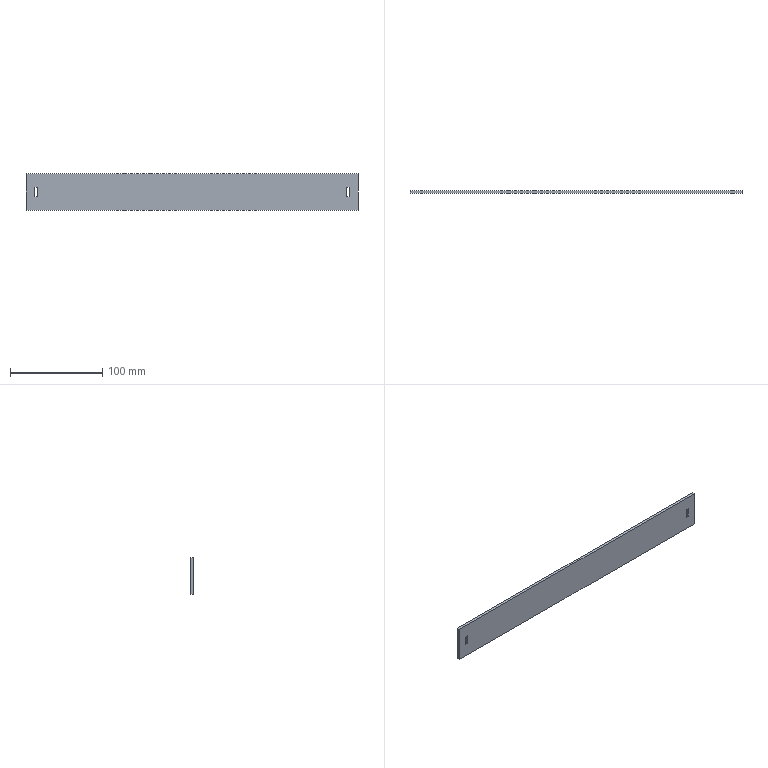Part | SolidWorks | features Extrusion 1, ICE 1 | 1 solid | 14 faces | box 360 x 3 x 40 mm | volume 43008 mm3 | plane 14
STEP:
#1=CARTESIAN_POINT('',(180.,0.,20.));
#2=VERTEX_POINT('',#1);
#3=CARTESIAN_POINT('',(180.,0.,-20.));
#4=VERTEX_POINT('',#3);
#5=CARTESIAN_POINT('',(180.,0.,20.));
#6=DIRECTION('',(0.,0.,-1.));
#7=VECTOR('',#6,1000.);
#8=LINE('',#5,#7);
#9=EDGE_CURVE('',#2,#4,#8,.T.);
#10=ORIENTED_EDGE('',*,*,#9,.T.);
#11=CARTESIAN_POINT('',(180.,3.,-20.));
#12=VERTEX_POINT('',#11);
#13=CARTESIAN_POINT('',(180.,3.,-20.));
#14=DIRECTION('',(0.,-1.,0.));
#15=VECTOR('',#14,1000.);
#16=LINE('',#13,#15);
#17=EDGE_CURVE('',#12,#4,#16,.T.);
#18=ORIENTED_EDGE('',*,*,#17,.F.);
#19=CARTESIAN_POINT('',(180.,3.,20.));
#20=VERTEX_POINT('',#19);
#21=CARTESIAN_POINT('',(180.,3.,20.));
#22=DIRECTION('',(0.,0.,-1.));
#23=VECTOR('',#22,1000.);
#24=LINE('',#21,#23);
#25=EDGE_CURVE('',#20,#12,#24,.T.);
#26=ORIENTED_EDGE('',*,*,#25,.F.);
#27=CARTESIAN_POINT('',(180.,3.,20.));
#28=DIRECTION('',(0.,-1.,0.));
#29=VECTOR('',#28,1000.);
#30=LINE('',#27,#29);
#31=EDGE_CURVE('',#20,#2,#30,.T.);
#32=ORIENTED_EDGE('',*,*,#31,.T.);
#33=EDGE_LOOP('',(#10,#18,#26,#32));
#34=FACE_OUTER_BOUND('',#33,.T.);
#35=CARTESIAN_POINT('',(180.,3.,20.));
#36=DIRECTION('',(-1.,0.,0.));
#37=DIRECTION('',(0.,0.,1.));
#38=AXIS2_PLACEMENT_3D('',#35,#36,#37);
#39=PLANE('',#38);
#40=ADVANCED_FACE('',(#34),#39,.F.);
#41=CARTESIAN_POINT('',(-180.,0.,-20.));
#42=VERTEX_POINT('',#41);
#43=CARTESIAN_POINT('',(-180.,0.,-20.));
#44=DIRECTION('',(-1.,0.,0.));
#45=VECTOR('',#44,1000.);
#46=LINE('',#43,#45);
#47=EDGE_CURVE('',#4,#42,#46,.T.);
#48=ORIENTED_EDGE('',*,*,#47,.T.);
#49=CARTESIAN_POINT('',(-180.,3.,-20.));
#50=VERTEX_POINT('',#49);
#51=CARTESIAN_POINT('',(-180.,3.,-20.));
#52=DIRECTION('',(0.,-1.,0.));
#53=VECTOR('',#52,1000.);
#54=LINE('',#51,#53);
#55=EDGE_CURVE('',#50,#42,#54,.T.);
#56=ORIENTED_EDGE('',*,*,#55,.F.);
#57=CARTESIAN_POINT('',(-180.,3.,-20.));
#58=DIRECTION('',(-1.,0.,0.));
#59=VECTOR('',#58,1000.);
#60=LINE('',#57,#59);
#61=EDGE_CURVE('',#12,#50,#60,.T.);
#62=ORIENTED_EDGE('',*,*,#61,.F.);
#63=ORIENTED_EDGE('',*,*,#17,.T.);
#64=EDGE_LOOP('',(#48,#56,#62,#63));
#65=FACE_OUTER_BOUND('',#64,.T.);
#66=CARTESIAN_POINT('',(-180.,3.,-20.));
#67=DIRECTION('',(0.,0.,1.));
#68=DIRECTION('',(1.,0.,0.));
#69=AXIS2_PLACEMENT_3D('',#66,#67,#68);
#70=PLANE('',#69);
#71=ADVANCED_FACE('',(#65),#70,.F.);
#72=CARTESIAN_POINT('',(-180.,0.,20.));
#73=VERTEX_POINT('',#72);
#74=CARTESIAN_POINT('',(-180.,0.,20.));
#75=DIRECTION('',(0.,0.,1.));
#76=VECTOR('',#75,1000.);
#77=LINE('',#74,#76);
#78=EDGE_CURVE('',#42,#73,#77,.T.);
#79=ORIENTED_EDGE('',*,*,#78,.T.);
#80=CARTESIAN_POINT('',(-180.,3.,20.));
#81=VERTEX_POINT('',#80);
#82=CARTESIAN_POINT('',(-180.,3.,20.));
#83=DIRECTION('',(0.,-1.,0.));
#84=VECTOR('',#83,1000.);
#85=LINE('',#82,#84);
#86=EDGE_CURVE('',#81,#73,#85,.T.);
#87=ORIENTED_EDGE('',*,*,#86,.F.);
#88=CARTESIAN_POINT('',(-180.,3.,20.));
#89=DIRECTION('',(0.,0.,1.));
#90=VECTOR('',#89,1000.);
#91=LINE('',#88,#90);
#92=EDGE_CURVE('',#50,#81,#91,.T.);
#93=ORIENTED_EDGE('',*,*,#92,.F.);
#94=ORIENTED_EDGE('',*,*,#55,.T.);
#95=EDGE_LOOP('',(#79,#87,#93,#94));
#96=FACE_OUTER_BOUND('',#95,.T.);
#97=CARTESIAN_POINT('',(-180.,3.,20.));
#98=DIRECTION('',(1.,0.,0.));
#99=DIRECTION('',(0.,0.,-1.));
#100=AXIS2_PLACEMENT_3D('',#97,#98,#99);
#101=PLANE('',#100);
#102=ADVANCED_FACE('',(#96),#101,.F.);
#103=CARTESIAN_POINT('',(-180.,0.,20.));
#104=DIRECTION('',(1.,0.,0.));
#105=VECTOR('',#104,1000.);
#106=LINE('',#103,#105);
#107=EDGE_CURVE('',#73,#2,#106,.T.);
#108=ORIENTED_EDGE('',*,*,#107,.T.);
#109=ORIENTED_EDGE('',*,*,#31,.F.);
#110=CARTESIAN_POINT('',(-180.,3.,20.));
#111=DIRECTION('',(1.,0.,0.));
#112=VECTOR('',#111,1000.);
#113=LINE('',#110,#112);
#114=EDGE_CURVE('',#81,#20,#113,.T.);
#115=ORIENTED_EDGE('',*,*,#114,.F.);
#116=ORIENTED_EDGE('',*,*,#86,.T.);
#117=EDGE_LOOP('',(#108,#109,#115,#116));
#118=FACE_OUTER_BOUND('',#117,.T.);
#119=CARTESIAN_POINT('',(-180.,3.,20.));
#120=DIRECTION('',(0.,0.,-1.));
#121=DIRECTION('',(-1.,0.,0.));
#122=AXIS2_PLACEMENT_3D('',#119,#120,#121);
#123=PLANE('',#122);
#124=ADVANCED_FACE('',(#118),#123,.F.);
#125=CARTESIAN_POINT('',(-170.6,3.,5.));
#126=VERTEX_POINT('',#125);
#127=CARTESIAN_POINT('',(-167.4,3.,5.));
#128=VERTEX_POINT('',#127);
#129=CARTESIAN_POINT('',(-170.6,3.,5.));
#130=DIRECTION('',(1.,0.,0.));
#131=VECTOR('',#130,1000.);
#132=LINE('',#129,#131);
#133=EDGE_CURVE('',#126,#128,#132,.T.);
#134=ORIENTED_EDGE('',*,*,#133,.F.);
#135=CARTESIAN_POINT('',(-170.6,3.,-5.));
#136=VERTEX_POINT('',#135);
#137=CARTESIAN_POINT('',(-170.6,3.,-5.));
#138=DIRECTION('',(0.,0.,1.));
#139=VECTOR('',#138,1000.);
#140=LINE('',#137,#139);
#141=EDGE_CURVE('',#136,#126,#140,.T.);
#142=ORIENTED_EDGE('',*,*,#141,.F.);
#143=CARTESIAN_POINT('',(-167.4,3.,-5.));
#144=VERTEX_POINT('',#143);
#145=CARTESIAN_POINT('',(-170.6,3.,-5.));
#146=DIRECTION('',(-1.,0.,0.));
#147=VECTOR('',#146,1000.);
#148=LINE('',#145,#147);
#149=EDGE_CURVE('',#144,#136,#148,.T.);
#150=ORIENTED_EDGE('',*,*,#149,.F.);
#151=CARTESIAN_POINT('',(-167.4,3.,-5.));
#152=DIRECTION('',(0.,0.,-1.));
#153=VECTOR('',#152,1000.);
#154=LINE('',#151,#153);
#155=EDGE_CURVE('',#128,#144,#154,.T.);
#156=ORIENTED_EDGE('',*,*,#155,.F.);
#157=EDGE_LOOP('',(#134,#142,#150,#156));
#158=FACE_BOUND('',#157,.T.);
#159=CARTESIAN_POINT('',(167.4,3.,-5.));
#160=VERTEX_POINT('',#159);
#161=CARTESIAN_POINT('',(167.4,3.,5.));
#162=VERTEX_POINT('',#161);
#163=CARTESIAN_POINT('',(167.4,3.,-5.));
#164=DIRECTION('',(0.,0.,1.));
#165=VECTOR('',#164,1000.);
#166=LINE('',#163,#165);
#167=EDGE_CURVE('',#160,#162,#166,.T.);
#168=ORIENTED_EDGE('',*,*,#167,.F.);
#169=CARTESIAN_POINT('',(170.6,3.,-5.));
#170=VERTEX_POINT('',#169);
#171=CARTESIAN_POINT('',(170.6,3.,-5.));
#172=DIRECTION('',(-1.,0.,0.));
#173=VECTOR('',#172,1000.);
#174=LINE('',#171,#173);
#175=EDGE_CURVE('',#170,#160,#174,.T.);
#176=ORIENTED_EDGE('',*,*,#175,.F.);
#177=CARTESIAN_POINT('',(170.6,3.,5.));
#178=VERTEX_POINT('',#177);
#179=CARTESIAN_POINT('',(170.6,3.,-5.));
#180=DIRECTION('',(0.,0.,-1.));
#181=VECTOR('',#180,1000.);
#182=LINE('',#179,#181);
#183=EDGE_CURVE('',#178,#170,#182,.T.);
#184=ORIENTED_EDGE('',*,*,#183,.F.);
#185=CARTESIAN_POINT('',(170.6,3.,5.));
#186=DIRECTION('',(1.,0.,0.));
#187=VECTOR('',#186,1000.);
#188=LINE('',#185,#187);
#189=EDGE_CURVE('',#162,#178,#188,.T.);
#190=ORIENTED_EDGE('',*,*,#189,.F.);
#191=EDGE_LOOP('',(#168,#176,#184,#190));
#192=FACE_BOUND('',#191,.T.);
#193=ORIENTED_EDGE('',*,*,#25,.T.);
#194=ORIENTED_EDGE('',*,*,#61,.T.);
#195=ORIENTED_EDGE('',*,*,#92,.T.);
#196=ORIENTED_EDGE('',*,*,#114,.T.);
#197=EDGE_LOOP('',(#193,#194,#195,#196));
#198=FACE_OUTER_BOUND('',#197,.T.);
#199=CARTESIAN_POINT('',(0.,3.,0.));
#200=DIRECTION('',(0.,-1.,0.));
#201=DIRECTION('',(0.,0.,-1.));
#202=AXIS2_PLACEMENT_3D('',#199,#200,#201);
#203=PLANE('',#202);
#204=ADVANCED_FACE('',(#158,#192,#198),#203,.F.);
#205=CARTESIAN_POINT('',(-170.6,0.,5.));
#206=VERTEX_POINT('',#205);
#207=CARTESIAN_POINT('',(-170.6,0.,-5.));
#208=VERTEX_POINT('',#207);
#209=CARTESIAN_POINT('',(-170.6,0.,0.));
#210=DIRECTION('',(0.,0.,-1.));
#211=VECTOR('',#210,1000.);
#212=LINE('',#209,#211);
#213=EDGE_CURVE('',#206,#208,#212,.T.);
#214=ORIENTED_EDGE('',*,*,#213,.F.);
#215=CARTESIAN_POINT('',(-167.4,0.,5.));
#216=VERTEX_POINT('',#215);
#217=CARTESIAN_POINT('',(0.,0.,5.));
#218=DIRECTION('',(-1.,0.,0.));
#219=VECTOR('',#218,1000.);
#220=LINE('',#217,#219);
#221=EDGE_CURVE('',#216,#206,#220,.T.);
#222=ORIENTED_EDGE('',*,*,#221,.F.);
#223=CARTESIAN_POINT('',(-167.4,0.,-5.));
#224=VERTEX_POINT('',#223);
#225=CARTESIAN_POINT('',(-167.4,0.,0.));
#226=DIRECTION('',(0.,0.,1.));
#227=VECTOR('',#226,1000.);
#228=LINE('',#225,#227);
#229=EDGE_CURVE('',#224,#216,#228,.T.);
#230=ORIENTED_EDGE('',*,*,#229,.F.);
#231=CARTESIAN_POINT('',(0.,0.,-5.));
#232=DIRECTION('',(1.,0.,0.));
#233=VECTOR('',#232,1000.);
#234=LINE('',#231,#233);
#235=EDGE_CURVE('',#208,#224,#234,.T.);
#236=ORIENTED_EDGE('',*,*,#235,.F.);
#237=EDGE_LOOP('',(#214,#222,#230,#236));
#238=FACE_BOUND('',#237,.T.);
#239=CARTESIAN_POINT('',(167.4,0.,-5.));
#240=VERTEX_POINT('',#239);
#241=CARTESIAN_POINT('',(170.6,0.,-5.));
#242=VERTEX_POINT('',#241);
#243=CARTESIAN_POINT('',(0.,0.,-5.));
#244=DIRECTION('',(1.,0.,0.));
#245=VECTOR('',#244,1000.);
#246=LINE('',#243,#245);
#247=EDGE_CURVE('',#240,#242,#246,.T.);
#248=ORIENTED_EDGE('',*,*,#247,.F.);
#249=CARTESIAN_POINT('',(167.4,0.,5.));
#250=VERTEX_POINT('',#249);
#251=CARTESIAN_POINT('',(167.4,0.,0.));
#252=DIRECTION('',(0.,0.,-1.));
#253=VECTOR('',#252,1000.);
#254=LINE('',#251,#253);
#255=EDGE_CURVE('',#250,#240,#254,.T.);
#256=ORIENTED_EDGE('',*,*,#255,.F.);
#257=CARTESIAN_POINT('',(170.6,0.,5.));
#258=VERTEX_POINT('',#257);
#259=CARTESIAN_POINT('',(0.,0.,5.));
#260=DIRECTION('',(-1.,0.,0.));
#261=VECTOR('',#260,1000.);
#262=LINE('',#259,#261);
#263=EDGE_CURVE('',#258,#250,#262,.T.);
#264=ORIENTED_EDGE('',*,*,#263,.F.);
#265=CARTESIAN_POINT('',(170.6,0.,0.));
#266=DIRECTION('',(0.,0.,1.));
#267=VECTOR('',#266,1000.);
#268=LINE('',#265,#267);
#269=EDGE_CURVE('',#242,#258,#268,.T.);
#270=ORIENTED_EDGE('',*,*,#269,.F.);
#271=EDGE_LOOP('',(#248,#256,#264,#270));
#272=FACE_BOUND('',#271,.T.);
#273=ORIENTED_EDGE('',*,*,#9,.F.);
#274=ORIENTED_EDGE('',*,*,#107,.F.);
#275=ORIENTED_EDGE('',*,*,#78,.F.);
#276=ORIENTED_EDGE('',*,*,#47,.F.);
#277=EDGE_LOOP('',(#273,#274,#275,#276));
#278=FACE_OUTER_BOUND('',#277,.T.);
#279=CARTESIAN_POINT('',(0.,0.,0.));
#280=DIRECTION('',(0.,-1.,0.));
#281=DIRECTION('',(0.,0.,-1.));
#282=AXIS2_PLACEMENT_3D('',#279,#280,#281);
#283=PLANE('',#282);
#284=ADVANCED_FACE('',(#238,#272,#278),#283,.T.);
#285=ORIENTED_EDGE('',*,*,#247,.T.);
#286=CARTESIAN_POINT('',(170.6,-7.,-5.));
#287=DIRECTION('',(0.,1.,0.));
#288=VECTOR('',#287,1000.);
#289=LINE('',#286,#288);
#290=EDGE_CURVE('',#242,#170,#289,.T.);
#291=ORIENTED_EDGE('',*,*,#290,.T.);
#292=ORIENTED_EDGE('',*,*,#175,.T.);
#293=CARTESIAN_POINT('',(167.4,-7.,-5.));
#294=DIRECTION('',(0.,1.,0.));
#295=VECTOR('',#294,1000.);
#296=LINE('',#293,#295);
#297=EDGE_CURVE('',#240,#160,#296,.T.);
#298=ORIENTED_EDGE('',*,*,#297,.F.);
#299=EDGE_LOOP('',(#285,#291,#292,#298));
#300=FACE_OUTER_BOUND('',#299,.T.);
#301=CARTESIAN_POINT('',(170.6,-7.,-5.));
#302=DIRECTION('',(0.,0.,-1.));
#303=DIRECTION('',(-1.,0.,0.));
#304=AXIS2_PLACEMENT_3D('',#301,#302,#303);
#305=PLANE('',#304);
#306=ADVANCED_FACE('',(#300),#305,.F.);
#307=ORIENTED_EDGE('',*,*,#269,.T.);
#308=CARTESIAN_POINT('',(170.6,-7.,5.));
#309=DIRECTION('',(0.,1.,0.));
#310=VECTOR('',#309,1000.);
#311=LINE('',#308,#310);
#312=EDGE_CURVE('',#258,#178,#311,.T.);
#313=ORIENTED_EDGE('',*,*,#312,.T.);
#314=ORIENTED_EDGE('',*,*,#183,.T.);
#315=ORIENTED_EDGE('',*,*,#290,.F.);
#316=EDGE_LOOP('',(#307,#313,#314,#315));
#317=FACE_OUTER_BOUND('',#316,.T.);
#318=CARTESIAN_POINT('',(170.6,-7.,-5.));
#319=DIRECTION('',(1.,0.,0.));
#320=DIRECTION('',(0.,0.,-1.));
#321=AXIS2_PLACEMENT_3D('',#318,#319,#320);
#322=PLANE('',#321);
#323=ADVANCED_FACE('',(#317),#322,.F.);
#324=ORIENTED_EDGE('',*,*,#263,.T.);
#325=CARTESIAN_POINT('',(167.4,-7.,5.));
#326=DIRECTION('',(0.,1.,0.));
#327=VECTOR('',#326,1000.);
#328=LINE('',#325,#327);
#329=EDGE_CURVE('',#250,#162,#328,.T.);
#330=ORIENTED_EDGE('',*,*,#329,.T.);
#331=ORIENTED_EDGE('',*,*,#189,.T.);
#332=ORIENTED_EDGE('',*,*,#312,.F.);
#333=EDGE_LOOP('',(#324,#330,#331,#332));
#334=FACE_OUTER_BOUND('',#333,.T.);
#335=CARTESIAN_POINT('',(170.6,-7.,5.));
#336=DIRECTION('',(0.,0.,1.));
#337=DIRECTION('',(1.,0.,0.));
#338=AXIS2_PLACEMENT_3D('',#335,#336,#337);
#339=PLANE('',#338);
#340=ADVANCED_FACE('',(#334),#339,.F.);
#341=ORIENTED_EDGE('',*,*,#255,.T.);
#342=ORIENTED_EDGE('',*,*,#297,.T.);
#343=ORIENTED_EDGE('',*,*,#167,.T.);
#344=ORIENTED_EDGE('',*,*,#329,.F.);
#345=EDGE_LOOP('',(#341,#342,#343,#344));
#346=FACE_OUTER_BOUND('',#345,.T.);
#347=CARTESIAN_POINT('',(167.4,-7.,-5.));
#348=DIRECTION('',(-1.,0.,0.));
#349=DIRECTION('',(0.,0.,1.));
#350=AXIS2_PLACEMENT_3D('',#347,#348,#349);
#351=PLANE('',#350);
#352=ADVANCED_FACE('',(#346),#351,.F.);
#353=ORIENTED_EDGE('',*,*,#213,.T.);
#354=CARTESIAN_POINT('',(-170.6,-7.,-5.));
#355=DIRECTION('',(0.,1.,0.));
#356=VECTOR('',#355,1000.);
#357=LINE('',#354,#356);
#358=EDGE_CURVE('',#208,#136,#357,.T.);
#359=ORIENTED_EDGE('',*,*,#358,.T.);
#360=ORIENTED_EDGE('',*,*,#141,.T.);
#361=CARTESIAN_POINT('',(-170.6,-7.,5.));
#362=DIRECTION('',(0.,1.,0.));
#363=VECTOR('',#362,1000.);
#364=LINE('',#361,#363);
#365=EDGE_CURVE('',#206,#126,#364,.T.);
#366=ORIENTED_EDGE('',*,*,#365,.F.);
#367=EDGE_LOOP('',(#353,#359,#360,#366));
#368=FACE_OUTER_BOUND('',#367,.T.);
#369=CARTESIAN_POINT('',(-170.6,-7.,-5.));
#370=DIRECTION('',(-1.,0.,0.));
#371=DIRECTION('',(0.,0.,1.));
#372=AXIS2_PLACEMENT_3D('',#369,#370,#371);
#373=PLANE('',#372);
#374=ADVANCED_FACE('',(#368),#373,.F.);
#375=ORIENTED_EDGE('',*,*,#235,.T.);
#376=CARTESIAN_POINT('',(-167.4,-7.,-5.));
#377=DIRECTION('',(0.,1.,0.));
#378=VECTOR('',#377,1000.);
#379=LINE('',#376,#378);
#380=EDGE_CURVE('',#224,#144,#379,.T.);
#381=ORIENTED_EDGE('',*,*,#380,.T.);
#382=ORIENTED_EDGE('',*,*,#149,.T.);
#383=ORIENTED_EDGE('',*,*,#358,.F.);
#384=EDGE_LOOP('',(#375,#381,#382,#383));
#385=FACE_OUTER_BOUND('',#384,.T.);
#386=CARTESIAN_POINT('',(-170.6,-7.,-5.));
#387=DIRECTION('',(0.,0.,-1.));
#388=DIRECTION('',(-1.,0.,0.));
#389=AXIS2_PLACEMENT_3D('',#386,#387,#388);
#390=PLANE('',#389);
#391=ADVANCED_FACE('',(#385),#390,.F.);
#392=ORIENTED_EDGE('',*,*,#229,.T.);
#393=CARTESIAN_POINT('',(-167.4,-7.,5.));
#394=DIRECTION('',(0.,1.,0.));
#395=VECTOR('',#394,1000.);
#396=LINE('',#393,#395);
#397=EDGE_CURVE('',#216,#128,#396,.T.);
#398=ORIENTED_EDGE('',*,*,#397,.T.);
#399=ORIENTED_EDGE('',*,*,#155,.T.);
#400=ORIENTED_EDGE('',*,*,#380,.F.);
#401=EDGE_LOOP('',(#392,#398,#399,#400));
#402=FACE_OUTER_BOUND('',#401,.T.);
#403=CARTESIAN_POINT('',(-167.4,-7.,-5.));
#404=DIRECTION('',(1.,0.,0.));
#405=DIRECTION('',(0.,0.,-1.));
#406=AXIS2_PLACEMENT_3D('',#403,#404,#405);
#407=PLANE('',#406);
#408=ADVANCED_FACE('',(#402),#407,.F.);
#409=ORIENTED_EDGE('',*,*,#221,.T.);
#410=ORIENTED_EDGE('',*,*,#365,.T.);
#411=ORIENTED_EDGE('',*,*,#133,.T.);
#412=ORIENTED_EDGE('',*,*,#397,.F.);
#413=EDGE_LOOP('',(#409,#410,#411,#412));
#414=FACE_OUTER_BOUND('',#413,.T.);
#415=CARTESIAN_POINT('',(-170.6,-7.,5.));
#416=DIRECTION('',(0.,0.,1.));
#417=DIRECTION('',(1.,0.,0.));
#418=AXIS2_PLACEMENT_3D('',#415,#416,#417);
#419=PLANE('',#418);
#420=ADVANCED_FACE('',(#414),#419,.F.);
#421=CLOSED_SHELL('',(#40,#71,#102,#124,#204,#284,#306,#323,#340,#352,#374,#391,#408,#420));
#422=MANIFOLD_SOLID_BREP('',#421);
#423=CARTESIAN_POINT('',(0.,0.,0.));
#424=DIRECTION('',(0.,0.,1.));
#425=DIRECTION('',(1.,0.,0.));
#426=AXIS2_PLACEMENT_3D('',#423,#424,#425);
#427=(LENGTH_UNIT()NAMED_UNIT(*)SI_UNIT(.MILLI.,.METRE.));
#428=UNCERTAINTY_MEASURE_WITH_UNIT(LENGTH_MEASURE(0.00001),#427,'','');
#429=(NAMED_UNIT(*)PLANE_ANGLE_UNIT()SI_UNIT($,.RADIAN.));
#430=(NAMED_UNIT(*)SI_UNIT($,.STERADIAN.)SOLID_ANGLE_UNIT());
#431=(GEOMETRIC_REPRESENTATION_CONTEXT(3)GLOBAL_UNCERTAINTY_ASSIGNED_CONTEXT((#428))GLOBAL_UNIT_ASSIGNED_CONTEXT((#427,#429,#430))REPRESENTATION_CONTEXT('',''));
#432=ADVANCED_BREP_SHAPE_REPRESENTATION('',(#422,#426),#431);